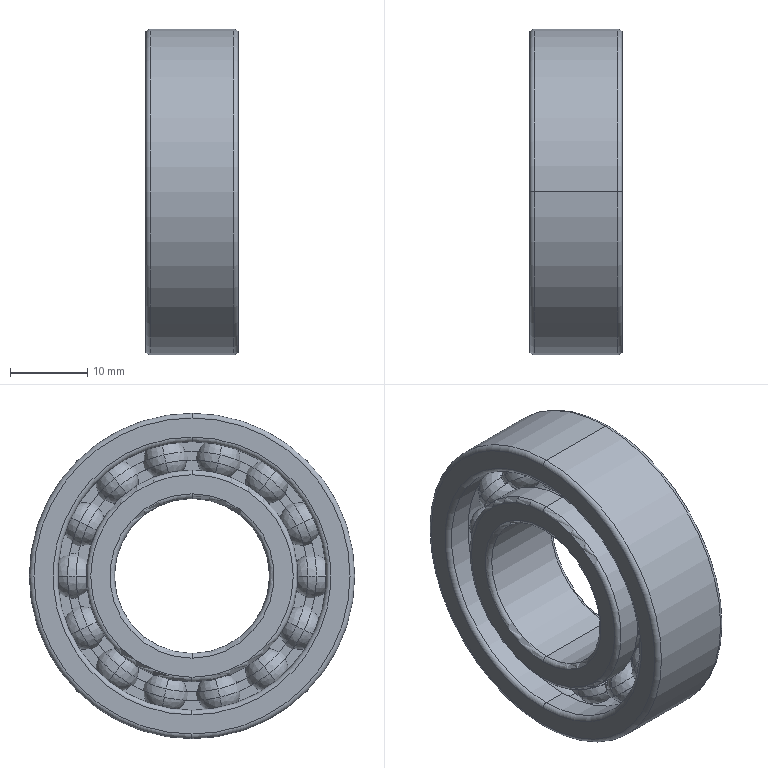Part | SolidWorks | features Revolution 5, CirPattern 2, RefAxis 1, RevCut 1 | 16 solids | 186 faces | box 12 x 42 x 42 mm | volume 9468 mm3 | cylinder 70 | sphere 60 | plane 34 | torus 20 | cone 2 | commonest cylinder face diameters 29.9 x27 32.1 x27 27.333 x4 34.667 x4 20 x2 24.889 x2